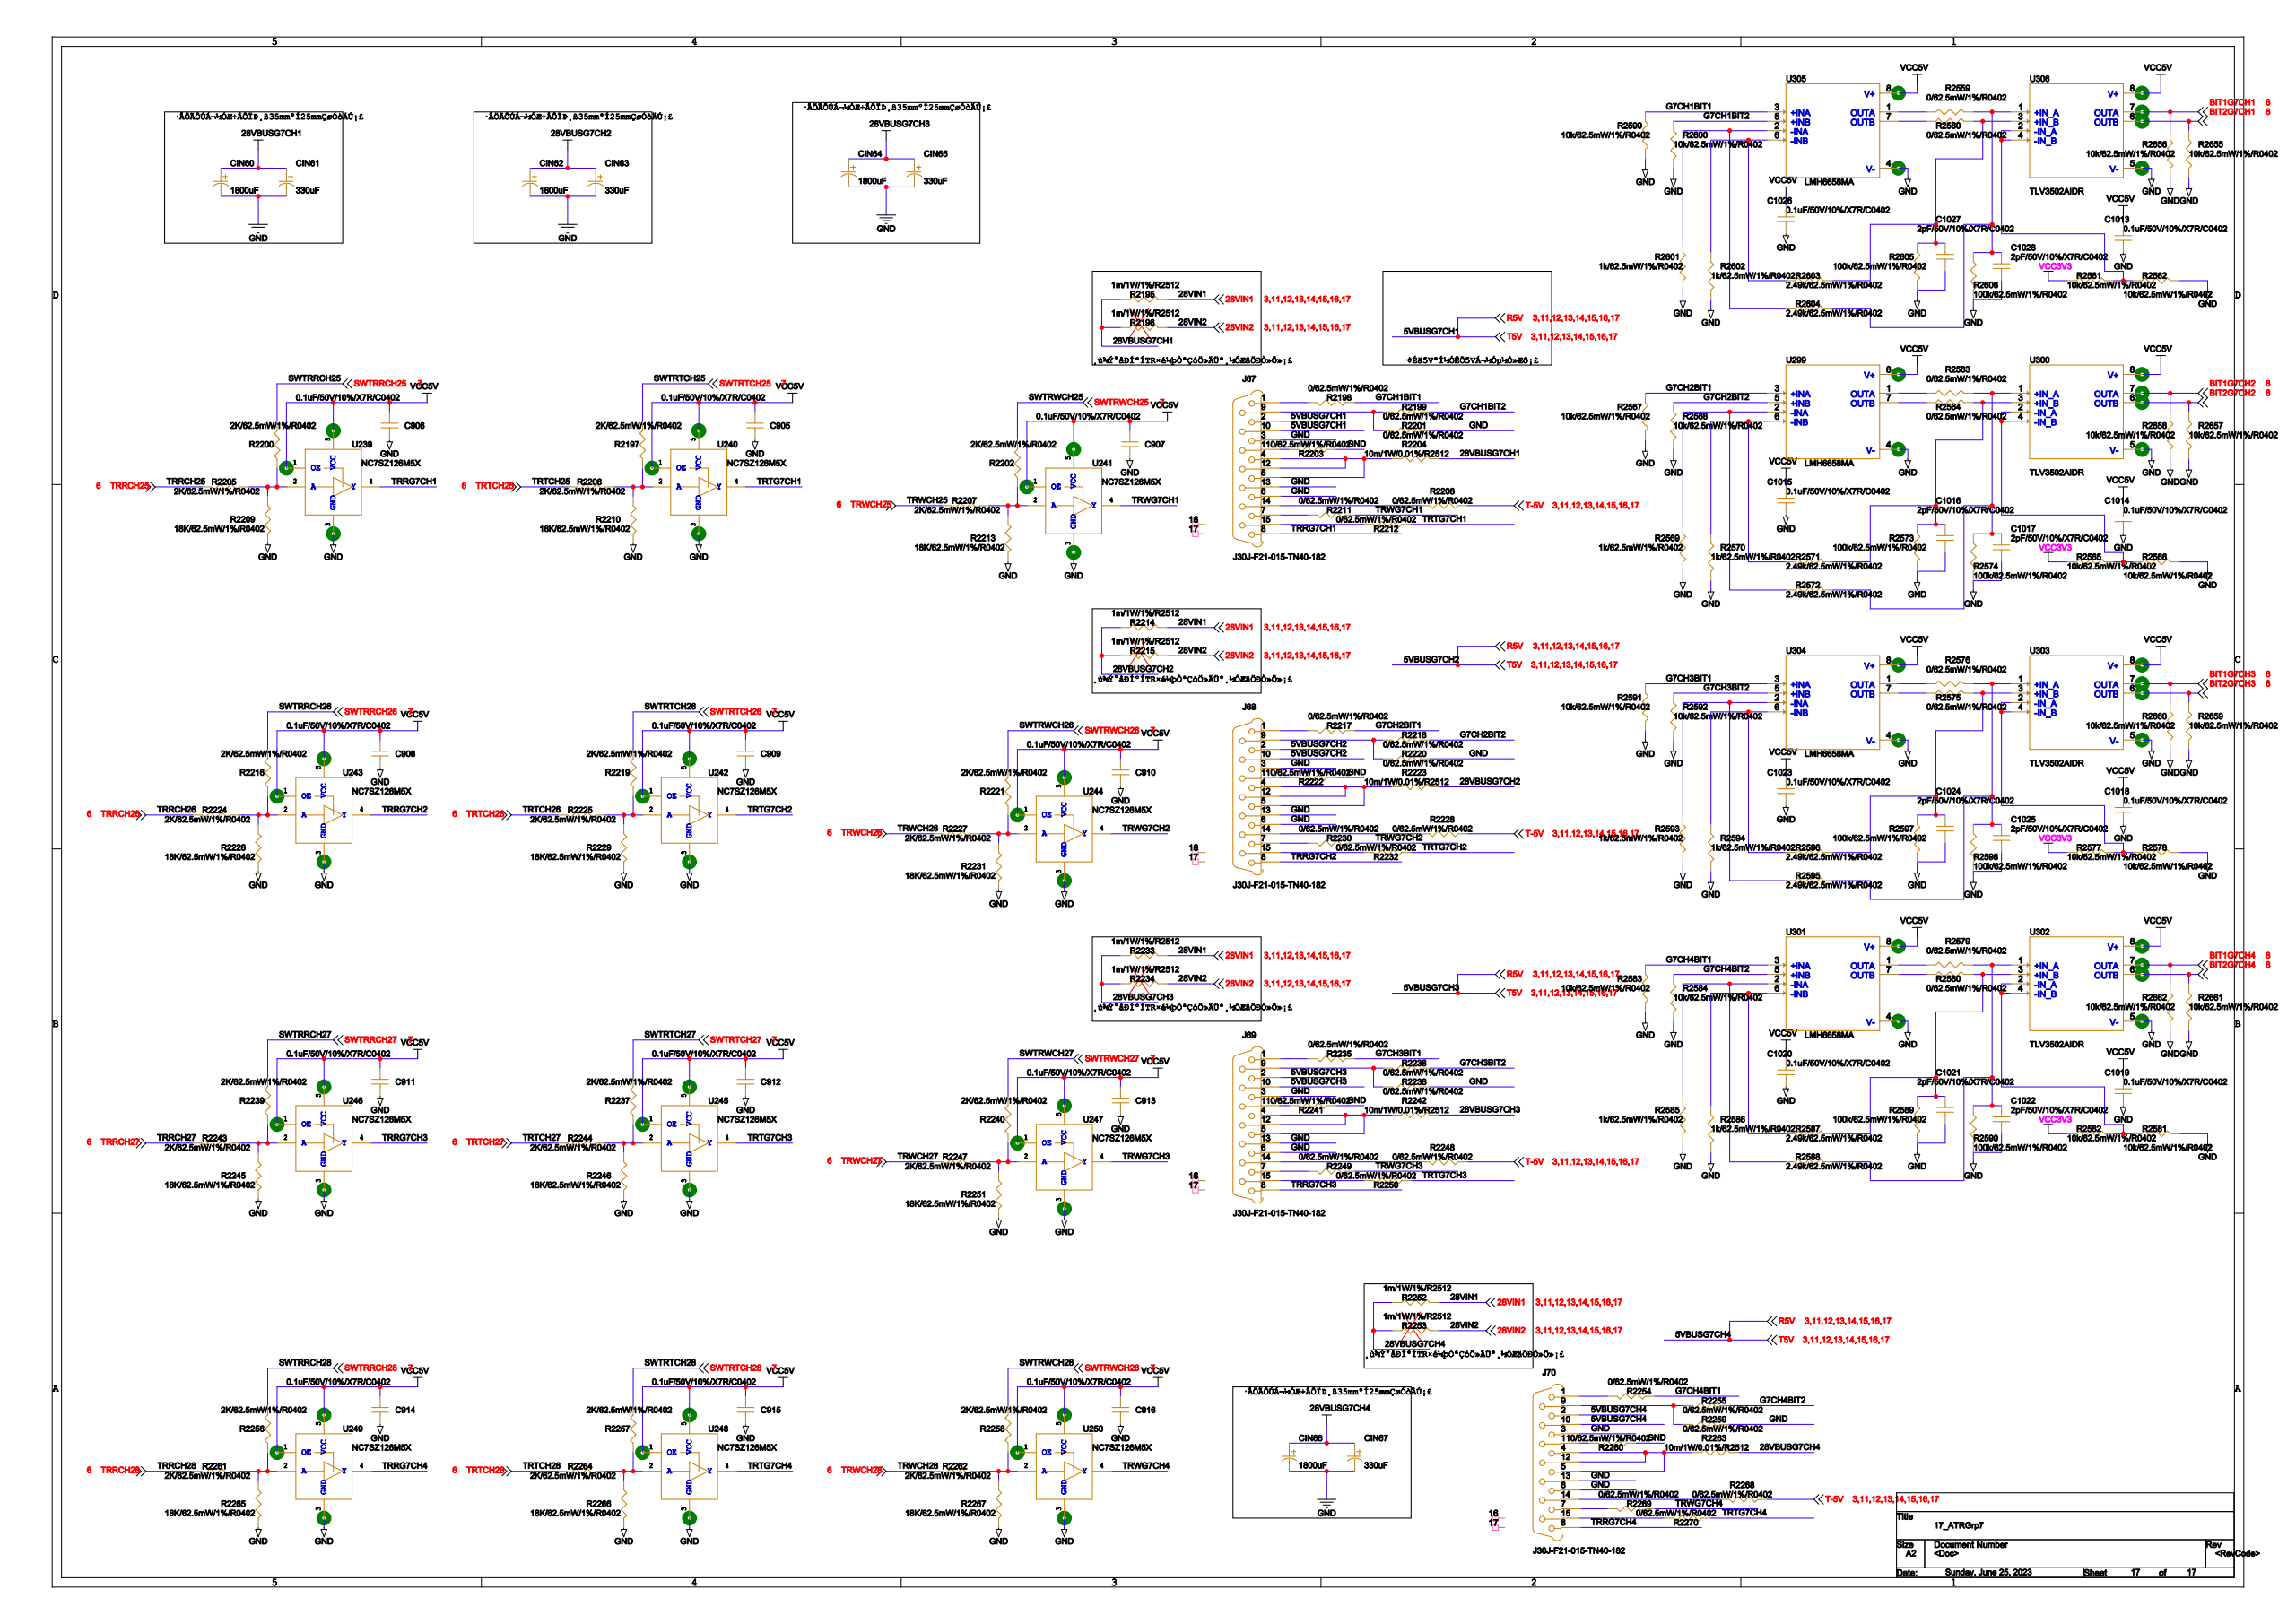Circuit board | Cadence Allegro | 2002 parts | 1538 nets | one sheet of the schematic
Parts on this sheet (reference | value | footprint):
C905 | 0.1uF/50V/10%/X7R/C0402 | 0402
C906 | 0.1uF/50V/10%/X7R/C0402 | 0402
C907 | 0.1uF/50V/10%/X7R/C0402 | 0402
C908 | 0.1uF/50V/10%/X7R/C0402 | 0402
C909 | 0.1uF/50V/10%/X7R/C0402 | 0402
C910 | 0.1uF/50V/10%/X7R/C0402 | 0402
C911 | 0.1uF/50V/10%/X7R/C0402 | 0402
C912 | 0.1uF/50V/10%/X7R/C0402 | 0402
C913 | 0.1uF/50V/10%/X7R/C0402 | 0402
C914 | 0.1uF/50V/10%/X7R/C0402 | 0402
C915 | 0.1uF/50V/10%/X7R/C0402 | 0402
C916 | 0.1uF/50V/10%/X7R/C0402 | 0402
C1013 | 0.1uF/50V/10%/X7R/C0402 | 0402
C1014 | 0.1uF/50V/10%/X7R/C0402 | 0402
C1016 | 2pF/50V/10%/X7R/C0402 | 0402
C1017 | 2pF/50V/10%/X7R/C0402 | 0402
C1018 | 0.1uF/50V/10%/X7R/C0402 | 0402
C1019 | 0.1uF/50V/10%/X7R/C0402 | 0402
C1021 | 2pF/50V/10%/X7R/C0402 | 0402
C1022 | 2pF/50V/10%/X7R/C0402 | 0402
C1024 | 2pF/50V/10%/X7R/C0402 | 0402
C1025 | 2pF/50V/10%/X7R/C0402 | 0402
C1027 | 2pF/50V/10%/X7R/C0402 | 0402
C1028 | 2pF/50V/10%/X7R/C0402 | 0402
CIN60 | ECF1HM182M27OTPO | AP-SMD_BD18-L27-W6_6-LS7_21
CIN61 | ECF1JM331G20OTPO | AP-SMD_BD10-L20-W6_6-LS7_21
CIN62 | ECF1HM182M27OTPO | AP-SMD_BD18-L27-W6_6-LS7_21
CIN63 | ECF1JM331G20OTPO | AP-SMD_BD10-L20-W6_6-LS7_21
CIN64 | ECF1HM182M27OTPO | AP-SMD_BD18-L27-W6_6-LS7_21
CIN65 | ECF1JM331G20OTPO | AP-SMD_BD10-L20-W6_6-LS7_21
CIN66 | ECF1HM182M27OTPO | AP-SMD_BD18-L27-W6_6-LS7_21
CIN67 | ECF1JM331G20OTPO | AP-SMD_BD10-L20-W6_6-LS7_21
J67 | J30J-F21-015-TN40-182 | J30J-F21-015-TN40-182
J68 | J30J-F21-015-TN40-182 | J30J-F21-015-TN40-182
J69 | J30J-F21-015-TN40-182 | J30J-F21-015-TN40-182
J70 | J30J-F21-015-TN40-182 | J30J-F21-015-TN40-182
R2195 | 1m/1W/1%/R2512 | 2512
R2196 | 1m/1W/1%/R2512 | 2512
R2197 | 2K/62.5mW/1%/R0402 | 0402
R2198 | 0/62.5mW/1%/R0402 | 0402
R2199 | 0/62.5mW/1%/R0402 | 0402
R2200 | 2K/62.5mW/1%/R0402 | 0402
R2201 | 0/62.5mW/1%/R0402 | 0402
R2202 | 2K/62.5mW/1%/R0402 | 0402
R2203 | 0/62.5mW/1%/R0402 | 0402
R2204 | 10m/1W/0.01%/R2512 | 2512
R2205 | 2K/62.5mW/1%/R0402 | 0402
R2206 | 2K/62.5mW/1%/R0402 | 0402
R2207 | 2K/62.5mW/1%/R0402 | 0402
R2208 | 0/62.5mW/1%/R0402 | 0402
R2209 | 18K/62.5mW/1%/R0402 | 0402
R2210 | 18K/62.5mW/1%/R0402 | 0402
R2211 | 0/62.5mW/1%/R0402 | 0402
R2212 | 0/62.5mW/1%/R0402 | 0402
R2213 | 18K/62.5mW/1%/R0402 | 0402
R2214 | 1m/1W/1%/R2512 | 2512
R2215 | 1m/1W/1%/R2512 | 2512
R2216 | 2K/62.5mW/1%/R0402 | 0402
R2217 | 0/62.5mW/1%/R0402 | 0402
R2218 | 0/62.5mW/1%/R0402 | 0402
R2219 | 2K/62.5mW/1%/R0402 | 0402
R2220 | 0/62.5mW/1%/R0402 | 0402
R2221 | 2K/62.5mW/1%/R0402 | 0402
R2222 | 0/62.5mW/1%/R0402 | 0402
R2223 | 10m/1W/0.01%/R2512 | 2512
R2224 | 2K/62.5mW/1%/R0402 | 0402
R2225 | 2K/62.5mW/1%/R0402 | 0402
R2226 | 18K/62.5mW/1%/R0402 | 0402
R2227 | 2K/62.5mW/1%/R0402 | 0402
R2228 | 0/62.5mW/1%/R0402 | 0402
R2229 | 18K/62.5mW/1%/R0402 | 0402
R2230 | 0/62.5mW/1%/R0402 | 0402
R2231 | 18K/62.5mW/1%/R0402 | 0402
R2232 | 0/62.5mW/1%/R0402 | 0402
R2233 | 1m/1W/1%/R2512 | 2512
R2234 | 1m/1W/1%/R2512 | 2512
R2235 | 0/62.5mW/1%/R0402 | 0402
R2236 | 0/62.5mW/1%/R0402 | 0402
R2237 | 2K/62.5mW/1%/R0402 | 0402
R2238 | 0/62.5mW/1%/R0402 | 0402
R2239 | 2K/62.5mW/1%/R0402 | 0402
R2240 | 2K/62.5mW/1%/R0402 | 0402
R2241 | 0/62.5mW/1%/R0402 | 0402
R2242 | 10m/1W/0.01%/R2512 | 2512
R2243 | 2K/62.5mW/1%/R0402 | 0402
R2244 | 2K/62.5mW/1%/R0402 | 0402
R2245 | 18K/62.5mW/1%/R0402 | 0402
R2246 | 18K/62.5mW/1%/R0402 | 0402
R2247 | 2K/62.5mW/1%/R0402 | 0402
R2248 | 0/62.5mW/1%/R0402 | 0402
R2249 | 0/62.5mW/1%/R0402 | 0402
R2250 | 0/62.5mW/1%/R0402 | 0402
R2251 | 18K/62.5mW/1%/R0402 | 0402
R2252 | 1m/1W/1%/R2512 | 2512
R2253 | 1m/1W/1%/R2512 | 2512
R2254 | 0/62.5mW/1%/R0402 | 0402
R2255 | 0/62.5mW/1%/R0402 | 0402
R2256 | 2K/62.5mW/1%/R0402 | 0402
R2257 | 2K/62.5mW/1%/R0402 | 0402
R2258 | 2K/62.5mW/1%/R0402 | 0402
R2259 | 0/62.5mW/1%/R0402 | 0402
R2260 | 0/62.5mW/1%/R0402 | 0402
R2261 | 2K/62.5mW/1%/R0402 | 0402
R2262 | 2K/62.5mW/1%/R0402 | 0402
R2263 | 10m/1W/0.01%/R2512 | 2512
R2264 | 2K/62.5mW/1%/R0402 | 0402
R2265 | 18K/62.5mW/1%/R0402 | 0402
R2266 | 18K/62.5mW/1%/R0402 | 0402
R2267 | 18K/62.5mW/1%/R0402 | 0402
R2268 | 0/62.5mW/1%/R0402 | 0402
R2269 | 0/62.5mW/1%/R0402 | 0402
R2270 | 0/62.5mW/1%/R0402 | 0402
R2559 | 0/62.5mW/1%/R0402 | 0402
R2560 | 0/62.5mW/1%/R0402 | 0402
R2561 | 10k/62.5mW/1%/R0402 | 0402
R2562 | 10k/62.5mW/1%/R0402 | 0402
R2563 | 0/62.5mW/1%/R0402 | 0402
R2564 | 0/62.5mW/1%/R0402 | 0402
R2565 | 10k/62.5mW/1%/R0402 | 0402
R2566 | 10k/62.5mW/1%/R0402 | 0402
R2567 | 10k/62.5mW/1%/R0402 | 0402
R2568 | 10k/62.5mW/1%/R0402 | 0402
R2569 | 1K/62.5mW/1%/R0402 | 0402
R2570 | 1K/62.5mW/1%/R0402 | 0402
R2572 | 2.49k/62.5mW/1%/R0402 | 0402
R2573 | 100k/62.5mW/1%/R0402 | 0402
R2574 | 100k/62.5mW/1%/R0402 | 0402
R2575 | 0/62.5mW/1%/R0402 | 0402
R2576 | 0/62.5mW/1%/R0402 | 0402
R2577 | 10k/62.5mW/1%/R0402 | 0402
R2578 | 10k/62.5mW/1%/R0402 | 0402
R2579 | 0/62.5mW/1%/R0402 | 0402
R2580 | 0/62.5mW/1%/R0402 | 0402
R2581 | 10k/62.5mW/1%/R0402 | 0402
R2582 | 10k/62.5mW/1%/R0402 | 0402
R2583 | 10k/62.5mW/1%/R0402 | 0402
R2584 | 10k/62.5mW/1%/R0402 | 0402
R2585 | 1K/62.5mW/1%/R0402 | 0402
R2586 | 1K/62.5mW/1%/R0402 | 0402
R2588 | 2.49k/62.5mW/1%/R0402 | 0402
R2589 | 100k/62.5mW/1%/R0402 | 0402
R2590 | 100k/62.5mW/1%/R0402 | 0402
R2591 | 10k/62.5mW/1%/R0402 | 0402
R2592 | 10k/62.5mW/1%/R0402 | 0402
R2593 | 1K/62.5mW/1%/R0402 | 0402
R2594 | 1K/62.5mW/1%/R0402 | 0402
R2595 | 2.49k/62.5mW/1%/R0402 | 0402
R2596 | 2.49k/62.5mW/1%/R0402 | 0402
R2597 | 100k/62.5mW/1%/R0402 | 0402
R2598 | 100k/62.5mW/1%/R0402 | 0402
R2599 | 10k/62.5mW/1%/R0402 | 0402
R2600 | 10k/62.5mW/1%/R0402 | 0402
R2601 | 1K/62.5mW/1%/R0402 | 0402
R2602 | 1K/62.5mW/1%/R0402 | 0402
R2604 | 2.49k/62.5mW/1%/R0402 | 0402
R2605 | 100k/62.5mW/1%/R0402 | 0402
R2606 | 100k/62.5mW/1%/R0402 | 0402
R2655 | 10k/62.5mW/1%/R0402 | 0402
R2656 | 10k/62.5mW/1%/R0402 | 0402
R2657 | 10k/62.5mW/1%/R0402 | 0402
R2658 | 10k/62.5mW/1%/R0402 | 0402
R2659 | 10k/62.5mW/1%/R0402 | 0402
R2660 | 10k/62.5mW/1%/R0402 | 0402
R2661 | 10k/62.5mW/1%/R0402 | 0402
R2662 | 10k/62.5mW/1%/R0402 | 0402
U239 | NC7SZ126M5X | SOT-23-5
U240 | NC7SZ126M5X | SOT-23-5
U241 | NC7SZ126M5X | SOT-23-5
U242 | NC7SZ126M5X | SOT-23-5
U243 | NC7SZ126M5X | SOT-23-5
U244 | NC7SZ126M5X | SOT-23-5
U245 | NC7SZ126M5X | SOT-23-5
U246 | NC7SZ126M5X | SOT-23-5
U247 | NC7SZ126M5X | SOT-23-5
U248 | NC7SZ126M5X | SOT-23-5
U249 | NC7SZ126M5X | SOT-23-5
U250 | NC7SZ126M5X | SOT-23-5
U299 | LMH6658MA | SOIC127P599X175-8N
U301 | LMH6658MA | SOIC127P599X175-8N
U303 | TLV3502AIDR | SOIC127P599X175-8N
U305 | LMH6658MA | SOIC127P599X175-8N
Nets of these parts (net: part-pin ...):
3.3V: R2561-1 R2565-1 R2577-1 R2582-1
AGND: C905-2 C906-2 C907-2 C908-2 C909-2 C910-2 C911-2 C912-2 C913-2 C914-2 C915-2 C916-2 C1013-2 C1014-2 C1016-2 C1017-2 C1018-2 C1019-2 C1021-2 C1022-2 C1024-2 C1025-2 C1027-2 C1028-2 CIN60-2 CIN61-2 CIN62-2 CIN63-2 CIN64-2 CIN65-2 CIN66-2 CIN67-2 J67-3 J67-6 J67-13 J68-3 J68-6 J68-13 J69-3 J69-6 J69-13 J70-3 J70-6 J70-13 R2201-1 R2203-1 R2209-1 R2210-1 R2213-1 R2220-1 R2222-1 R2226-1 R2229-1 R2231-1 R2238-1 R2241-1 R2245-1 R2246-1 R2251-1 R2259-1 R2260-1 R2265-1 R2266-1 R2267-1 R2562-2 R2566-2 R2567-2 R2568-2 R2569-2 R2570-2 R2573-2 R2574-2 R2578-2 R2581-2 R2583-2 R2584-2 R2585-2 R2586-2 R2589-2 R2590-2 R2591-2 R2592-2 R2593-2 R2594-2 R2597-2 R2598-2 R2599-2 R2600-2 R2601-2 R2602-2 R2605-2 R2606-2 R2655-2 R2656-2 R2657-2 R2658-2 R2659-2 R2660-2 R2661-2 R2662-2 U239-3 U240-3 U241-3 U242-3 U243-3 U244-3 U245-3 U246-3 U247-3 U248-3 U249-3 U250-3 U299-4 U301-4 U303-5 U305-4
VCC5V: C905-1 C906-1 C907-1 C908-1 C909-1 C910-1 C911-1 C912-1 C913-1 C914-1 C915-1 C916-1 C1013-1 C1014-1 C1018-1 C1019-1 U239-1 U239-5 U240-1 U240-5 U241-1 U241-5 U242-1 U242-5 U243-1 U243-5 U244-1 U244-5 U245-1 U245-5 U246-1 U246-5 U247-1 U247-5 U248-1 U248-5 U249-1 U249-5 U250-1 U250-5 U299-8 U301-8 U303-8 U305-8
28VIN1: R2195-2 R2196-2 R2214-2 R2215-2 R2233-2 R2234-2 R2252-2 R2253-2
R5V: J67-2 J67-10 J68-2 J68-10 J69-2 J69-10 J70-2 J70-10
T-5V: R2208-1 R2228-1 R2248-1 R2268-1
N24412987: R2570-1 U299-6
N24412997: C1016-1 R2564-2 R2573-1
N24412975: R2569-1 R2572-1 U299-2
N24412995: C1017-1 R2563-2 R2572-2 R2574-1
N24413541: R2586-1 U301-6
N24413551: C1021-1 R2580-2 R2589-1
N24413529: R2585-1 R2588-1 U301-2
N24413549: C1022-1 R2579-2 R2588-2 R2590-1
N24413353: R2593-1 R2595-1
N24413369: C1025-1 R2576-2 R2595-2 R2598-1 U303-1
N24413357: R2594-1 R2596-1
N24413371: C1024-1 R2575-2 R2596-2 R2597-1 U303-3
N24412807: R2602-1 U305-6
N24412817: C1027-1 R2560-2 R2605-1
N24412803: R2601-1 R2604-1 U305-2
N24412815: C1028-1 R2559-2 R2604-2 R2606-1
G7CH2BIT1: R2217-1 R2567-1 U299-3
G7CH2BIT2: R2218-1 R2568-1 U299-5
N24412991: R2563-1 U299-1
N24412993: R2564-1 U299-7
G7CH4BIT1: R2254-1 R2583-1 U301-3
G7CH4BIT2: R2255-1 R2584-1 U301-5
N24413545: R2579-1 U301-1
N24413547: R2580-1 U301-7
G7CH3BIT1: R2235-1 R2591-1
G7CH3BIT2: R2236-1 R2592-1
N24413365: R2576-1
N24413367: R2575-1
G7CH1BIT1: R2198-1 R2599-1 U305-3
G7CH1BIT2: R2199-1 R2600-1 U305-5
N24412811: R2559-1 U305-1
N24412813: R2560-1 U305-7
N24413049: R2565-2 R2566-1
BIT1G7CH2: R2658-1
BIT2G7CH2: R2657-1
N24413603: R2581-1 R2582-2
BIT1G7CH4: R2662-1
BIT2G7CH4: R2661-1
N24413423: R2577-2 R2578-1 U303-2 U303-4
BIT1G7CH3: R2660-1 U303-7
BIT2G7CH3: R2659-1 U303-6
N24412869: R2561-2 R2562-1
BIT1G7CH1: R2656-1
BIT2G7CH1: R2655-1
N23736092: J67-1 R2198-2
N23736105: J67-11 R2203-2
N23736107: J67-4 J67-5 J67-12 R2204-1
N23736119: J67-14 R2208-2
N23736123: J67-15 R2212-2
N23736121: J67-7 R2211-2
TRRG7CH1: J67-8 U239-4
N23736094: J67-9 R2199-2 R2201-2
N23736651: J68-1 R2217-2
N23736664: J68-11 R2222-2
N23736666: J68-4 J68-5 J68-12 R2223-1
N23736678: J68-14 R2228-2
N23736682: J68-15 R2232-2
N23736680: J68-7 R2230-2
TRRG7CH2: J68-8 U243-4
N23736653: J68-9 R2218-2 R2220-2
N23737278: J69-1 R2235-2
N23737291: J69-11 R2241-2
N23737293: J69-4 J69-5 J69-12 R2242-1
N23737305: J69-14 R2248-2
N23737309: J69-15 R2250-2
N23737307: J69-7 R2249-2
TRRG7CH3: J69-8 U246-4
N23737280: J69-9 R2236-2 R2238-2
N23737910: J70-1 R2254-2
N23737923: J70-11 R2260-2
N23737925: J70-4 J70-5 J70-12 R2263-1
N23737937: J70-14 R2268-2
N23737941: J70-15 R2270-2
N23737939: J70-7 R2269-2
TRRG7CH4: J70-8 U249-4
N23737912: J70-9 R2255-2 R2259-2
28VBUSG7CH1: CIN60-1 CIN61-1 R2195-1 R2196-1 R2204-2
28VBUSG7CH2: CIN62-1 CIN63-1 R2214-1 R2215-1 R2223-2
28VBUSG7CH3: CIN64-1 CIN65-1 R2233-1 R2234-1 R2242-2
28VBUSG7CH4: CIN66-1 CIN67-1 R2252-1 R2253-1 R2263-2
SWTRTCH25: R2197-1
N24020874: R2197-2 R2206-2 R2210-2 U240-2
SWTRRCH25: R2200-1
N24021854: R2200-2 R2205-2 R2209-2 U239-2
SWTRWCH25: R2202-1
N24021362: R2202-2 R2207-2 R2213-2 U241-2
TRRCH25: R2205-1
TRTCH25: R2206-1
TRWCH25: R2207-1
SWTRRCH26: R2216-1
N24021972: R2216-2 R2224-2 R2226-2 U243-2
SWTRTCH26: R2219-1
N24020992: R2219-2 R2225-2 R2229-2 U242-2
SWTRWCH26: R2221-1
N24021484: R2221-2 R2227-2 R2231-2 U244-2
TRRCH26: R2224-1
TRTCH26: R2225-1
TRWCH26: R2227-1
SWTRTCH27: R2237-1
N24021118: R2237-2 R2244-2 R2246-2 U245-2
SWTRRCH27: R2239-1
N24022098: R2239-2 R2243-2 R2245-2 U246-2
SWTRWCH27: R2240-1
N24021606: R2240-2 R2247-2 R2251-2 U247-2
TRRCH27: R2243-1
TRTCH27: R2244-1
TRWCH27: R2247-1
SWTRRCH28: R2256-1
N24022216: R2256-2 R2261-2 R2265-2 U249-2
SWTRTCH28: R2257-1
N24021240: R2257-2 R2264-2 R2266-2 U248-2
SWTRWCH28: R2258-1
N24021728: R2258-2 R2262-2 R2267-2 U250-2
TRRCH28: R2261-1
TRWCH28: R2262-1
TRTCH28: R2264-1
TRTG7CH1: R2212-1 U240-4
TRWG7CH1: R2211-1 U241-4
TRTG7CH2: R2232-1 U242-4
TRWG7CH2: R2230-1 U244-4
TRTG7CH3: R2250-1 U245-4
TRWG7CH3: R2249-1 U247-4
TRTG7CH4: R2270-1 U248-4
TRWG7CH4: R2269-1 U250-4